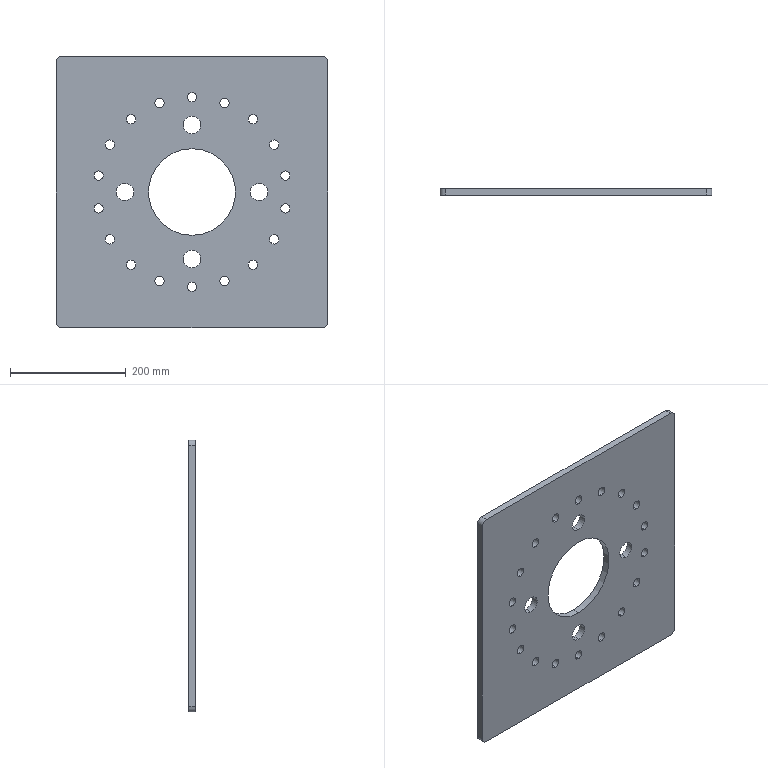Part | SolidWorks | features HoleWzd 2, Extrusion 1 | 1 solid | 56 faces | box 470 x 12 x 470 mm | volume 2360354 mm3 | cylinder 50 | plane 6 | commonest cylinder face diameters 16 x36 30 x8 20 x4 150 x2